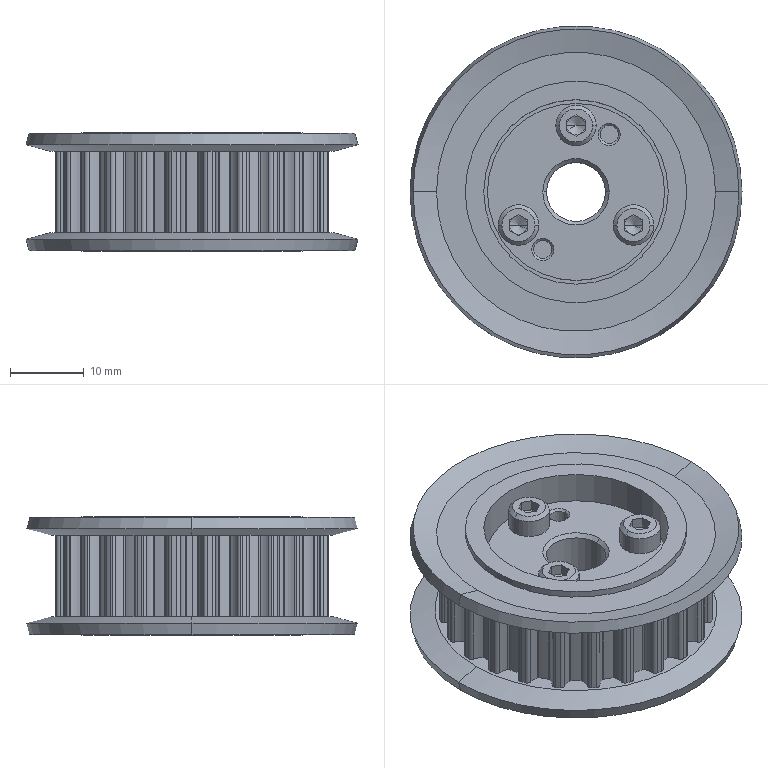Part | STEP file | ECC05-S5M100-24-F-d8 stepper motor timing pulley | 1 solid | 346 faces | box 45 x 45 x 16 mm | volume 14077 mm3 | cylinder 245 | plane 51 | cone 50 | commonest cylinder face diameters 1.1 x58 0.5 x56 6.55 x50 33.7 x25 37.24 x24 2.459 x16